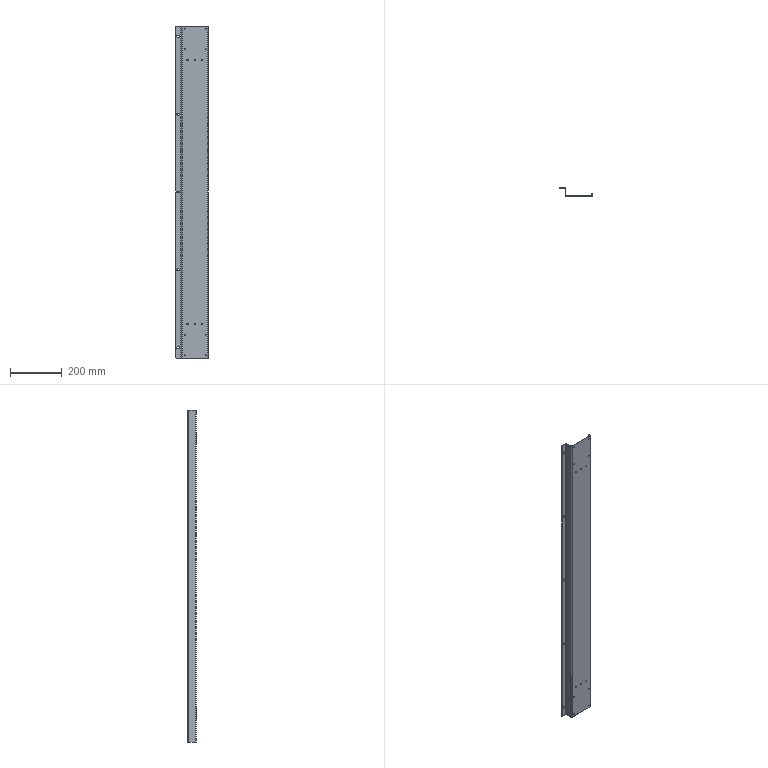Part | NX | features BREP 1 | 1 solid | 82 faces | box 127 x 32 x 1280 mm | volume 411517 mm3 | cylinder 44 | plane 38 | commonest cylinder face diameters 3.3 x16 5 x12 6.6 x10 4 x3 8 x3